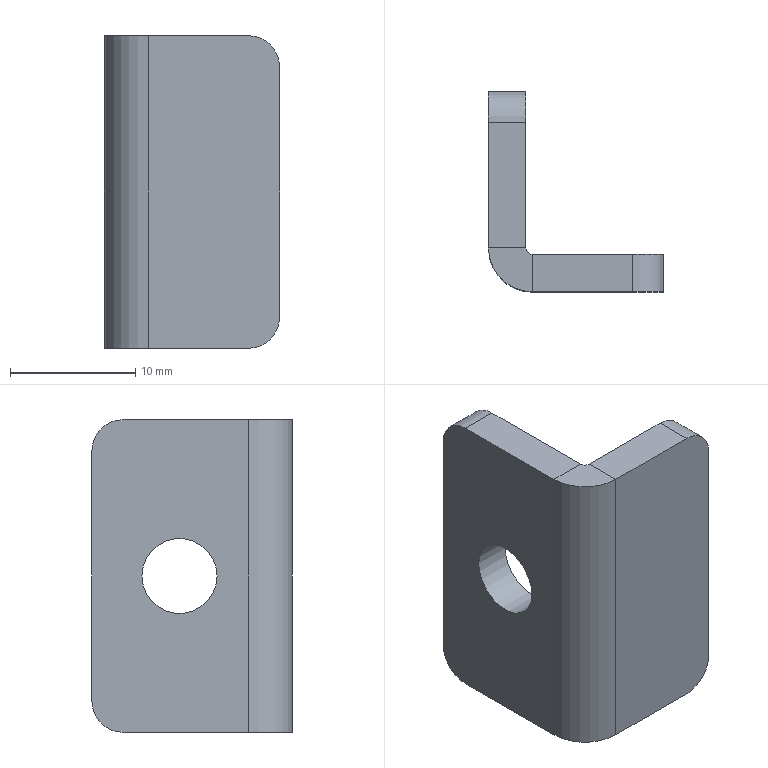Part | STEP file | 6100513 | 1 solid | 19 faces | box 14 x 16 x 25 mm | volume 1860 mm3 | plane 12 | cylinder 7 | commonest cylinder face diameters 5 x4 1 x1 6 x1 7 x1
STEP:
#1=CARTESIAN_POINT('',(0.,0.,0.));
#2=DIRECTION('',(0.,0.,1.));
#3=DIRECTION('',(1.,0.,0.));
#4=AXIS2_PLACEMENT_3D('',#1,#2,#3);
#5=CARTESIAN_POINT('',(0.,3.5,12.5));
#6=VERTEX_POINT('',#5);
#7=CARTESIAN_POINT('',(3.,3.5,12.5));
#8=VERTEX_POINT('',#7);
#9=CARTESIAN_POINT('',(0.,3.5,12.5));
#10=DIRECTION('',(1.,0.,0.));
#11=VECTOR('',#10,1.);
#12=LINE('',#9,#11);
#13=CARTESIAN_POINT('',(0.,3.5,12.5));
#14=DIRECTION('',(0.,0.,1.));
#15=DIRECTION('',(1.,0.,0.));
#16=AXIS2_PLACEMENT_3D('',#13,#14,#15);
#17=PLANE('',#16);
#18=CARTESIAN_POINT('',(0.,0.));
#19=DIRECTION('',(1.,0.));
#20=VECTOR('',#19,1.);
#21=LINE('',#18,#20);
#22=(GEOMETRIC_REPRESENTATION_CONTEXT(2)PARAMETRIC_REPRESENTATION_CONTEXT()REPRESENTATION_CONTEXT('',''));
#23=DEFINITIONAL_REPRESENTATION('',(#21),#22);
#24=PCURVE('',#17,#23);
#25=CARTESIAN_POINT('',(3.5,3.,12.5));
#26=DIRECTION('',(0.,0.,1.));
#27=DIRECTION('',(1.,0.,0.));
#28=AXIS2_PLACEMENT_3D('',#25,#26,#27);
#29=PLANE('',#28);
#30=CARTESIAN_POINT('',(-3.5,0.5));
#31=DIRECTION('',(1.,0.));
#32=VECTOR('',#31,1.);
#33=LINE('',#30,#32);
#34=(GEOMETRIC_REPRESENTATION_CONTEXT(2)PARAMETRIC_REPRESENTATION_CONTEXT()REPRESENTATION_CONTEXT('',''));
#35=DEFINITIONAL_REPRESENTATION('',(#33),#34);
#36=PCURVE('',#29,#35);
#37=SURFACE_CURVE('',#12,(#24,#36),.PCURVE_S1.);
#38=EDGE_CURVE('',#6,#8,#37,.T.);
#39=ORIENTED_EDGE('',*,*,#38,.F.);
#40=CARTESIAN_POINT('',(3.5,0.,12.5));
#41=VERTEX_POINT('',#40);
#42=CARTESIAN_POINT('',(3.5,3.5,12.5));
#43=DIRECTION('',(0.,0.,1.));
#44=DIRECTION('',(-1.,0.,0.));
#45=AXIS2_PLACEMENT_3D('',#42,#43,#44);
#46=CIRCLE('',#45,3.5);
#47=CARTESIAN_POINT('',(3.5,0.));
#48=DIRECTION('',(-1.,0.));
#49=AXIS2_PLACEMENT_2D('',#47,#48);
#50=CIRCLE('',#49,3.5);
#51=(GEOMETRIC_REPRESENTATION_CONTEXT(2)PARAMETRIC_REPRESENTATION_CONTEXT()REPRESENTATION_CONTEXT('',''));
#52=DEFINITIONAL_REPRESENTATION('',(#50),#51);
#53=PCURVE('',#17,#52);
#54=CARTESIAN_POINT('',(3.5,3.5,12.5));
#55=DIRECTION('',(0.,0.,-1.));
#56=DIRECTION('',(-1.,0.,0.));
#57=AXIS2_PLACEMENT_3D('',#54,#55,#56);
#58=CYLINDRICAL_SURFACE('',#57,3.5);
#59=CARTESIAN_POINT('',(6.283,0.));
#60=DIRECTION('',(-1.,0.));
#61=VECTOR('',#60,1.);
#62=LINE('',#59,#61);
#63=(GEOMETRIC_REPRESENTATION_CONTEXT(2)PARAMETRIC_REPRESENTATION_CONTEXT()REPRESENTATION_CONTEXT('',''));
#64=DEFINITIONAL_REPRESENTATION('',(#62),#63);
#65=PCURVE('',#58,#64);
#66=SURFACE_CURVE('',#46,(#53,#65),.PCURVE_S1.);
#67=EDGE_CURVE('',#6,#41,#66,.T.);
#68=ORIENTED_EDGE('',*,*,#67,.T.);
#69=CARTESIAN_POINT('',(3.5,3.,12.5));
#70=VERTEX_POINT('',#69);
#71=CARTESIAN_POINT('',(3.5,3.,12.5));
#72=DIRECTION('',(0.,-1.,0.));
#73=VECTOR('',#72,1.);
#74=LINE('',#71,#73);
#75=CARTESIAN_POINT('',(3.5,-0.5));
#76=DIRECTION('',(0.,-1.));
#77=VECTOR('',#76,1.);
#78=LINE('',#75,#77);
#79=(GEOMETRIC_REPRESENTATION_CONTEXT(2)PARAMETRIC_REPRESENTATION_CONTEXT()REPRESENTATION_CONTEXT('',''));
#80=DEFINITIONAL_REPRESENTATION('',(#78),#79);
#81=PCURVE('',#17,#80);
#82=CARTESIAN_POINT('',(3.5,3.5,12.5));
#83=DIRECTION('',(0.,0.,1.));
#84=DIRECTION('',(1.,0.,0.));
#85=AXIS2_PLACEMENT_3D('',#82,#83,#84);
#86=PLANE('',#85);
#87=CARTESIAN_POINT('',(0.,-0.5));
#88=DIRECTION('',(0.,-1.));
#89=VECTOR('',#88,1.);
#90=LINE('',#87,#89);
#91=(GEOMETRIC_REPRESENTATION_CONTEXT(2)PARAMETRIC_REPRESENTATION_CONTEXT()REPRESENTATION_CONTEXT('',''));
#92=DEFINITIONAL_REPRESENTATION('',(#90),#91);
#93=PCURVE('',#86,#92);
#94=SURFACE_CURVE('',#74,(#81,#93),.PCURVE_S1.);
#95=EDGE_CURVE('',#70,#41,#94,.T.);
#96=ORIENTED_EDGE('',*,*,#95,.F.);
#97=CARTESIAN_POINT('',(3.5,3.5,12.5));
#98=DIRECTION('',(0.,0.,1.));
#99=DIRECTION('',(1.,0.,0.));
#100=AXIS2_PLACEMENT_3D('',#97,#98,#99);
#101=CIRCLE('',#100,0.5);
#102=CARTESIAN_POINT('',(3.5,0.));
#103=DIRECTION('',(1.,0.));
#104=AXIS2_PLACEMENT_2D('',#102,#103);
#105=CIRCLE('',#104,0.5);
#106=(GEOMETRIC_REPRESENTATION_CONTEXT(2)PARAMETRIC_REPRESENTATION_CONTEXT()REPRESENTATION_CONTEXT('',''));
#107=DEFINITIONAL_REPRESENTATION('',(#105),#106);
#108=PCURVE('',#17,#107);
#109=CARTESIAN_POINT('',(3.5,3.5,12.5));
#110=DIRECTION('',(0.,0.,-1.));
#111=DIRECTION('',(-1.,0.,0.));
#112=AXIS2_PLACEMENT_3D('',#109,#110,#111);
#113=CYLINDRICAL_SURFACE('',#112,0.5);
#114=CARTESIAN_POINT('',(9.425,0.));
#115=DIRECTION('',(-1.,0.));
#116=VECTOR('',#115,1.);
#117=LINE('',#114,#116);
#118=(GEOMETRIC_REPRESENTATION_CONTEXT(2)PARAMETRIC_REPRESENTATION_CONTEXT()REPRESENTATION_CONTEXT('',''));
#119=DEFINITIONAL_REPRESENTATION('',(#117),#118);
#120=PCURVE('',#113,#119);
#121=SURFACE_CURVE('',#101,(#108,#120),.PCURVE_S1.);
#122=EDGE_CURVE('',#8,#70,#121,.T.);
#123=ORIENTED_EDGE('',*,*,#122,.F.);
#124=EDGE_LOOP('',(#39,#68,#96,#123));
#125=FACE_BOUND('',#124,.T.);
#126=ADVANCED_FACE('',(#125),#17,.T.);
#127=CARTESIAN_POINT('',(3.,13.5,12.5));
#128=VERTEX_POINT('',#127);
#129=CARTESIAN_POINT('',(3.,16.,12.5));
#130=DIRECTION('',(0.,-1.,0.));
#131=VECTOR('',#130,1.);
#132=LINE('',#129,#131);
#133=CARTESIAN_POINT('',(-0.5,13.));
#134=DIRECTION('',(0.,-1.));
#135=VECTOR('',#134,1.);
#136=LINE('',#133,#135);
#137=(GEOMETRIC_REPRESENTATION_CONTEXT(2)PARAMETRIC_REPRESENTATION_CONTEXT()REPRESENTATION_CONTEXT('',''));
#138=DEFINITIONAL_REPRESENTATION('',(#136),#137);
#139=PCURVE('',#29,#138);
#140=CARTESIAN_POINT('',(3.,16.,12.5));
#141=DIRECTION('',(1.,0.,0.));
#142=DIRECTION('',(0.,1.,0.));
#143=AXIS2_PLACEMENT_3D('',#140,#141,#142);
#144=PLANE('',#143);
#145=CARTESIAN_POINT('',(0.,0.));
#146=DIRECTION('',(-1.,0.));
#147=VECTOR('',#146,1.);
#148=LINE('',#145,#147);
#149=(GEOMETRIC_REPRESENTATION_CONTEXT(2)PARAMETRIC_REPRESENTATION_CONTEXT()REPRESENTATION_CONTEXT('',''));
#150=DEFINITIONAL_REPRESENTATION('',(#148),#149);
#151=PCURVE('',#144,#150);
#152=SURFACE_CURVE('',#132,(#139,#151),.PCURVE_S1.);
#153=EDGE_CURVE('',#128,#8,#152,.T.);
#154=ORIENTED_EDGE('',*,*,#153,.F.);
#155=CARTESIAN_POINT('',(0.,13.5,12.5));
#156=VERTEX_POINT('',#155);
#157=CARTESIAN_POINT('',(3.5,13.5,12.5));
#158=DIRECTION('',(-1.,0.,0.));
#159=VECTOR('',#158,1.);
#160=LINE('',#157,#159);
#161=CARTESIAN_POINT('',(0.,10.5));
#162=DIRECTION('',(-1.,0.));
#163=VECTOR('',#162,1.);
#164=LINE('',#161,#163);
#165=(GEOMETRIC_REPRESENTATION_CONTEXT(2)PARAMETRIC_REPRESENTATION_CONTEXT()REPRESENTATION_CONTEXT('',''));
#166=DEFINITIONAL_REPRESENTATION('',(#164),#165);
#167=PCURVE('',#29,#166);
#168=CARTESIAN_POINT('',(0.,13.5,10.));
#169=DIRECTION('',(1.,0.,0.));
#170=DIRECTION('',(0.,1.,0.));
#171=AXIS2_PLACEMENT_3D('',#168,#169,#170);
#172=CYLINDRICAL_SURFACE('',#171,2.5);
#173=CARTESIAN_POINT('',(1.571,3.5));
#174=DIRECTION('',(0.,-1.));
#175=VECTOR('',#174,1.);
#176=LINE('',#173,#175);
#177=(GEOMETRIC_REPRESENTATION_CONTEXT(2)PARAMETRIC_REPRESENTATION_CONTEXT()REPRESENTATION_CONTEXT('',''));
#178=DEFINITIONAL_REPRESENTATION('',(#176),#177);
#179=PCURVE('',#172,#178);
#180=SURFACE_CURVE('',#160,(#167,#179),.PCURVE_S1.);
#181=EDGE_CURVE('',#128,#156,#180,.T.);
#182=ORIENTED_EDGE('',*,*,#181,.T.);
#183=CARTESIAN_POINT('',(0.,16.,12.5));
#184=DIRECTION('',(0.,-1.,0.));
#185=VECTOR('',#184,1.);
#186=LINE('',#183,#185);
#187=CARTESIAN_POINT('',(-3.5,13.));
#188=DIRECTION('',(0.,-1.));
#189=VECTOR('',#188,1.);
#190=LINE('',#187,#189);
#191=(GEOMETRIC_REPRESENTATION_CONTEXT(2)PARAMETRIC_REPRESENTATION_CONTEXT()REPRESENTATION_CONTEXT('',''));
#192=DEFINITIONAL_REPRESENTATION('',(#190),#191);
#193=PCURVE('',#29,#192);
#194=CARTESIAN_POINT('',(0.,16.,12.5));
#195=DIRECTION('',(1.,0.,0.));
#196=DIRECTION('',(0.,1.,0.));
#197=AXIS2_PLACEMENT_3D('',#194,#195,#196);
#198=PLANE('',#197);
#199=CARTESIAN_POINT('',(0.,0.));
#200=DIRECTION('',(-1.,0.));
#201=VECTOR('',#200,1.);
#202=LINE('',#199,#201);
#203=(GEOMETRIC_REPRESENTATION_CONTEXT(2)PARAMETRIC_REPRESENTATION_CONTEXT()REPRESENTATION_CONTEXT('',''));
#204=DEFINITIONAL_REPRESENTATION('',(#202),#203);
#205=PCURVE('',#198,#204);
#206=SURFACE_CURVE('',#186,(#193,#205),.PCURVE_S1.);
#207=EDGE_CURVE('',#156,#6,#206,.T.);
#208=ORIENTED_EDGE('',*,*,#207,.T.);
#209=ORIENTED_EDGE('',*,*,#38,.T.);
#210=EDGE_LOOP('',(#154,#182,#208,#209));
#211=FACE_BOUND('',#210,.T.);
#212=ADVANCED_FACE('',(#211),#29,.T.);
#213=CARTESIAN_POINT('',(3.5,0.,-12.5));
#214=VERTEX_POINT('',#213);
#215=CARTESIAN_POINT('',(3.5,3.,-12.5));
#216=VERTEX_POINT('',#215);
#217=CARTESIAN_POINT('',(3.5,0.,-12.5));
#218=DIRECTION('',(0.,1.,0.));
#219=VECTOR('',#218,1.);
#220=LINE('',#217,#219);
#221=CARTESIAN_POINT('',(3.5,0.,-12.5));
#222=DIRECTION('',(0.,0.,-1.));
#223=DIRECTION('',(-1.,0.,0.));
#224=AXIS2_PLACEMENT_3D('',#221,#222,#223);
#225=PLANE('',#224);
#226=CARTESIAN_POINT('',(0.,0.));
#227=DIRECTION('',(0.,1.));
#228=VECTOR('',#227,1.);
#229=LINE('',#226,#228);
#230=(GEOMETRIC_REPRESENTATION_CONTEXT(2)PARAMETRIC_REPRESENTATION_CONTEXT()REPRESENTATION_CONTEXT('',''));
#231=DEFINITIONAL_REPRESENTATION('',(#229),#230);
#232=PCURVE('',#225,#231);
#233=CARTESIAN_POINT('',(3.,3.5,-12.5));
#234=DIRECTION('',(0.,0.,-1.));
#235=DIRECTION('',(-1.,0.,0.));
#236=AXIS2_PLACEMENT_3D('',#233,#234,#235);
#237=PLANE('',#236);
#238=CARTESIAN_POINT('',(-0.5,-3.5));
#239=DIRECTION('',(0.,1.));
#240=VECTOR('',#239,1.);
#241=LINE('',#238,#240);
#242=(GEOMETRIC_REPRESENTATION_CONTEXT(2)PARAMETRIC_REPRESENTATION_CONTEXT()REPRESENTATION_CONTEXT('',''));
#243=DEFINITIONAL_REPRESENTATION('',(#241),#242);
#244=PCURVE('',#237,#243);
#245=SURFACE_CURVE('',#220,(#232,#244),.PCURVE_S1.);
#246=EDGE_CURVE('',#214,#216,#245,.T.);
#247=ORIENTED_EDGE('',*,*,#246,.F.);
#248=CARTESIAN_POINT('',(0.,3.5,-12.5));
#249=VERTEX_POINT('',#248);
#250=CARTESIAN_POINT('',(3.5,3.5,-12.5));
#251=DIRECTION('',(0.,0.,1.));
#252=DIRECTION('',(-1.,0.,0.));
#253=AXIS2_PLACEMENT_3D('',#250,#251,#252);
#254=CIRCLE('',#253,3.5);
#255=CARTESIAN_POINT('',(3.5,3.5));
#256=CARTESIAN_POINT('',(3.5,-2.562));
#257=CARTESIAN_POINT('',(-1.75,0.4689));
#258=CARTESIAN_POINT('',(-7.,3.5));
#259=CARTESIAN_POINT('',(-1.75,6.531));
#260=CARTESIAN_POINT('',(3.5,9.562));
#261=CARTESIAN_POINT('',(3.5,3.5));
#262=(BOUNDED_CURVE()B_SPLINE_CURVE(2,(#255,#256,#257,#258,#259,#260,#261),.UNSPECIFIED.,.T.,.F.)B_SPLINE_CURVE_WITH_KNOTS((1,2,2,2,2,1),(-2.094,0.,2.094,4.189,6.283,8.378),.UNSPECIFIED.)CURVE()GEOMETRIC_REPRESENTATION_ITEM()RATIONAL_B_SPLINE_CURVE((1.,0.5,1.,0.5,1.,0.5,1.))REPRESENTATION_ITEM(''));
#263=(GEOMETRIC_REPRESENTATION_CONTEXT(2)PARAMETRIC_REPRESENTATION_CONTEXT()REPRESENTATION_CONTEXT('',''));
#264=DEFINITIONAL_REPRESENTATION('',(#262),#263);
#265=PCURVE('',#225,#264);
#266=CARTESIAN_POINT('',(6.283,25.));
#267=DIRECTION('',(-1.,0.));
#268=VECTOR('',#267,1.);
#269=LINE('',#266,#268);
#270=(GEOMETRIC_REPRESENTATION_CONTEXT(2)PARAMETRIC_REPRESENTATION_CONTEXT()REPRESENTATION_CONTEXT('',''));
#271=DEFINITIONAL_REPRESENTATION('',(#269),#270);
#272=PCURVE('',#58,#271);
#273=SURFACE_CURVE('',#254,(#265,#272),.PCURVE_S1.);
#274=EDGE_CURVE('',#249,#214,#273,.T.);
#275=ORIENTED_EDGE('',*,*,#274,.F.);
#276=CARTESIAN_POINT('',(3.,3.5,-12.5));
#277=VERTEX_POINT('',#276);
#278=CARTESIAN_POINT('',(3.,3.5,-12.5));
#279=DIRECTION('',(-1.,0.,0.));
#280=VECTOR('',#279,1.);
#281=LINE('',#278,#280);
#282=CARTESIAN_POINT('',(0.5,3.5));
#283=DIRECTION('',(1.,0.));
#284=VECTOR('',#283,1.);
#285=LINE('',#282,#284);
#286=(GEOMETRIC_REPRESENTATION_CONTEXT(2)PARAMETRIC_REPRESENTATION_CONTEXT()REPRESENTATION_CONTEXT('',''));
#287=DEFINITIONAL_REPRESENTATION('',(#285),#286);
#288=PCURVE('',#225,#287);
#289=CARTESIAN_POINT('',(3.5,3.5,-12.5));
#290=DIRECTION('',(0.,0.,1.));
#291=DIRECTION('',(1.,0.,0.));
#292=AXIS2_PLACEMENT_3D('',#289,#290,#291);
#293=PLANE('',#292);
#294=CARTESIAN_POINT('',(-0.5,0.));
#295=DIRECTION('',(-1.,0.));
#296=VECTOR('',#295,1.);
#297=LINE('',#294,#296);
#298=(GEOMETRIC_REPRESENTATION_CONTEXT(2)PARAMETRIC_REPRESENTATION_CONTEXT()REPRESENTATION_CONTEXT('',''));
#299=DEFINITIONAL_REPRESENTATION('',(#297),#298);
#300=PCURVE('',#293,#299);
#301=SURFACE_CURVE('',#281,(#288,#300),.PCURVE_S1.);
#302=EDGE_CURVE('',#277,#249,#301,.T.);
#303=ORIENTED_EDGE('',*,*,#302,.F.);
#304=CARTESIAN_POINT('',(3.5,3.5,-12.5));
#305=DIRECTION('',(0.,0.,1.));
#306=DIRECTION('',(1.,0.,0.));
#307=AXIS2_PLACEMENT_3D('',#304,#305,#306);
#308=CIRCLE('',#307,0.5);
#309=CARTESIAN_POINT('',(-0.5,3.5));
#310=CARTESIAN_POINT('',(-0.5,4.366));
#311=CARTESIAN_POINT('',(0.25,3.933));
#312=CARTESIAN_POINT('',(1.,3.5));
#313=CARTESIAN_POINT('',(0.25,3.067));
#314=CARTESIAN_POINT('',(-0.5,2.634));
#315=CARTESIAN_POINT('',(-0.5,3.5));
#316=(BOUNDED_CURVE()B_SPLINE_CURVE(2,(#309,#310,#311,#312,#313,#314,#315),.UNSPECIFIED.,.T.,.F.)B_SPLINE_CURVE_WITH_KNOTS((1,2,2,2,2,1),(-2.094,0.,2.094,4.189,6.283,8.378),.UNSPECIFIED.)CURVE()GEOMETRIC_REPRESENTATION_ITEM()RATIONAL_B_SPLINE_CURVE((1.,0.5,1.,0.5,1.,0.5,1.))REPRESENTATION_ITEM(''));
#317=(GEOMETRIC_REPRESENTATION_CONTEXT(2)PARAMETRIC_REPRESENTATION_CONTEXT()REPRESENTATION_CONTEXT('',''));
#318=DEFINITIONAL_REPRESENTATION('',(#316),#317);
#319=PCURVE('',#225,#318);
#320=CARTESIAN_POINT('',(9.425,25.));
#321=DIRECTION('',(-1.,0.));
#322=VECTOR('',#321,1.);
#323=LINE('',#320,#322);
#324=(GEOMETRIC_REPRESENTATION_CONTEXT(2)PARAMETRIC_REPRESENTATION_CONTEXT()REPRESENTATION_CONTEXT('',''));
#325=DEFINITIONAL_REPRESENTATION('',(#323),#324);
#326=PCURVE('',#113,#325);
#327=SURFACE_CURVE('',#308,(#319,#326),.PCURVE_S1.);
#328=EDGE_CURVE('',#277,#216,#327,.T.);
#329=ORIENTED_EDGE('',*,*,#328,.T.);
#330=EDGE_LOOP('',(#247,#275,#303,#329));
#331=FACE_BOUND('',#330,.T.);
#332=ADVANCED_FACE('',(#331),#225,.T.);
#333=CARTESIAN_POINT('',(11.5,3.,-12.5));
#334=VERTEX_POINT('',#333);
#335=CARTESIAN_POINT('',(3.5,3.,-12.5));
#336=DIRECTION('',(1.,0.,0.));
#337=VECTOR('',#336,1.);
#338=LINE('',#335,#337);
#339=CARTESIAN_POINT('',(-0.5,-0.5));
#340=DIRECTION('',(-1.,0.));
#341=VECTOR('',#340,1.);
#342=LINE('',#339,#341);
#343=(GEOMETRIC_REPRESENTATION_CONTEXT(2)PARAMETRIC_REPRESENTATION_CONTEXT()REPRESENTATION_CONTEXT('',''));
#344=DEFINITIONAL_REPRESENTATION('',(#342),#343);
#345=PCURVE('',#237,#344);
#346=CARTESIAN_POINT('',(3.5,3.,12.5));
#347=DIRECTION('',(0.,1.,0.));
#348=DIRECTION('',(0.,0.,1.));
#349=AXIS2_PLACEMENT_3D('',#346,#347,#348);
#350=PLANE('',#349);
#351=CARTESIAN_POINT('',(-25.,0.));
#352=DIRECTION('',(0.,1.));
#353=VECTOR('',#352,1.);
#354=LINE('',#351,#353);
#355=(GEOMETRIC_REPRESENTATION_CONTEXT(2)PARAMETRIC_REPRESENTATION_CONTEXT()REPRESENTATION_CONTEXT('',''));
#356=DEFINITIONAL_REPRESENTATION('',(#354),#355);
#357=PCURVE('',#350,#356);
#358=SURFACE_CURVE('',#338,(#345,#357),.PCURVE_S1.);
#359=EDGE_CURVE('',#216,#334,#358,.T.);
#360=ORIENTED_EDGE('',*,*,#359,.T.);
#361=CARTESIAN_POINT('',(11.5,0.,-12.5));
#362=VERTEX_POINT('',#361);
#363=CARTESIAN_POINT('',(11.5,3.5,-12.5));
#364=DIRECTION('',(0.,-1.,0.));
#365=VECTOR('',#364,1.);
#366=LINE('',#363,#365);
#367=CARTESIAN_POINT('',(-8.5,0.));
#368=DIRECTION('',(0.,-1.));
#369=VECTOR('',#368,1.);
#370=LINE('',#367,#369);
#371=(GEOMETRIC_REPRESENTATION_CONTEXT(2)PARAMETRIC_REPRESENTATION_CONTEXT()REPRESENTATION_CONTEXT('',''));
#372=DEFINITIONAL_REPRESENTATION('',(#370),#371);
#373=PCURVE('',#237,#372);
#374=CARTESIAN_POINT('',(11.5,3.5,-10.));
#375=DIRECTION('',(0.,-1.,0.));
#376=DIRECTION('',(0.,0.,-1.));
#377=AXIS2_PLACEMENT_3D('',#374,#375,#376);
#378=CYLINDRICAL_SURFACE('',#377,2.5);
#379=CARTESIAN_POINT('',(0.,0.));
#380=DIRECTION('',(0.,1.));
#381=VECTOR('',#380,1.);
#382=LINE('',#379,#381);
#383=(GEOMETRIC_REPRESENTATION_CONTEXT(2)PARAMETRIC_REPRESENTATION_CONTEXT()REPRESENTATION_CONTEXT('',''));
#384=DEFINITIONAL_REPRESENTATION('',(#382),#383);
#385=PCURVE('',#378,#384);
#386=SURFACE_CURVE('',#366,(#373,#385),.PCURVE_S1.);
#387=EDGE_CURVE('',#334,#362,#386,.T.);
#388=ORIENTED_EDGE('',*,*,#387,.T.);
#389=CARTESIAN_POINT('',(3.5,0.,-12.5));
#390=DIRECTION('',(1.,0.,0.));
#391=VECTOR('',#390,1.);
#392=LINE('',#389,#391);
#393=CARTESIAN_POINT('',(-0.5,-3.5));
#394=DIRECTION('',(-1.,0.));
#395=VECTOR('',#394,1.);
#396=LINE('',#393,#395);
#397=(GEOMETRIC_REPRESENTATION_CONTEXT(2)PARAMETRIC_REPRESENTATION_CONTEXT()REPRESENTATION_CONTEXT('',''));
#398=DEFINITIONAL_REPRESENTATION('',(#396),#397);
#399=PCURVE('',#237,#398);
#400=CARTESIAN_POINT('',(3.5,0.,12.5));
#401=DIRECTION('',(0.,1.,0.));
#402=DIRECTION('',(0.,0.,1.));
#403=AXIS2_PLACEMENT_3D('',#400,#401,#402);
#404=PLANE('',#403);
#405=CARTESIAN_POINT('',(-25.,0.));
#406=DIRECTION('',(0.,1.));
#407=VECTOR('',#406,1.);
#408=LINE('',#405,#407);
#409=(GEOMETRIC_REPRESENTATION_CONTEXT(2)PARAMETRIC_REPRESENTATION_CONTEXT()REPRESENTATION_CONTEXT('',''));
#410=DEFINITIONAL_REPRESENTATION('',(#408),#409);
#411=PCURVE('',#404,#410);
#412=SURFACE_CURVE('',#392,(#399,#411),.PCURVE_S1.);
#413=EDGE_CURVE('',#214,#362,#412,.T.);
#414=ORIENTED_EDGE('',*,*,#413,.F.);
#415=ORIENTED_EDGE('',*,*,#246,.T.);
#416=EDGE_LOOP('',(#360,#388,#414,#415));
#417=FACE_BOUND('',#416,.T.);
#418=ADVANCED_FACE('',(#417),#237,.T.);
#419=ORIENTED_EDGE('',*,*,#413,.T.);
#420=CARTESIAN_POINT('',(14.,0.,-10.));
#421=VERTEX_POINT('',#420);
#422=CARTESIAN_POINT('',(11.5,0.,-10.));
#423=DIRECTION('',(0.,-1.,0.));
#424=DIRECTION('',(0.,0.,1.));
#425=AXIS2_PLACEMENT_3D('',#422,#423,#424);
#426=CIRCLE('',#425,2.5);
#427=CARTESIAN_POINT('',(-20.,8.));
#428=CARTESIAN_POINT('',(-20.,3.67));
#429=CARTESIAN_POINT('',(-23.75,5.835));
#430=CARTESIAN_POINT('',(-27.5,8.));
#431=CARTESIAN_POINT('',(-23.75,10.165));
#432=CARTESIAN_POINT('',(-20.,12.33));
#433=CARTESIAN_POINT('',(-20.,8.));
#434=(BOUNDED_CURVE()B_SPLINE_CURVE(2,(#427,#428,#429,#430,#431,#432,#433),.UNSPECIFIED.,.T.,.F.)B_SPLINE_CURVE_WITH_KNOTS((1,2,2,2,2,1),(-2.094,0.,2.094,4.189,6.283,8.378),.UNSPECIFIED.)CURVE()GEOMETRIC_REPRESENTATION_ITEM()RATIONAL_B_SPLINE_CURVE((1.,0.5,1.,0.5,1.,0.5,1.))REPRESENTATION_ITEM(''));
#435=(GEOMETRIC_REPRESENTATION_CONTEXT(2)PARAMETRIC_REPRESENTATION_CONTEXT()REPRESENTATION_CONTEXT('',''));
#436=DEFINITIONAL_REPRESENTATION('',(#434),#435);
#437=PCURVE('',#404,#436);
#438=CARTESIAN_POINT('',(-3.142,3.5));
#439=DIRECTION('',(1.,0.));
#440=VECTOR('',#439,1.);
#441=LINE('',#438,#440);
#442=(GEOMETRIC_REPRESENTATION_CONTEXT(2)PARAMETRIC_REPRESENTATION_CONTEXT()REPRESENTATION_CONTEXT('',''));
#443=DEFINITIONAL_REPRESENTATION('',(#441),#442);
#444=PCURVE('',#378,#443);
#445=SURFACE_CURVE('',#426,(#437,#444),.PCURVE_S1.);
#446=EDGE_CURVE('',#362,#421,#445,.T.);
#447=ORIENTED_EDGE('',*,*,#446,.T.);
#448=CARTESIAN_POINT('',(14.,0.,10.));
#449=VERTEX_POINT('',#448);
#450=CARTESIAN_POINT('',(14.,0.,12.5));
#451=DIRECTION('',(0.,0.,-1.));
#452=VECTOR('',#451,1.);
#453=LINE('',#450,#452);
#454=CARTESIAN_POINT('',(0.,10.5));
#455=DIRECTION('',(-1.,0.));
#456=VECTOR('',#455,1.);
#457=LINE('',#454,#456);
#458=(GEOMETRIC_REPRESENTATION_CONTEXT(2)PARAMETRIC_REPRESENTATION_CONTEXT()REPRESENTATION_CONTEXT('',''));
#459=DEFINITIONAL_REPRESENTATION('',(#457),#458);
#460=PCURVE('',#404,#459);
#461=CARTESIAN_POINT('',(14.,3.,12.5));
#462=DIRECTION('',(1.,0.,0.));
#463=DIRECTION('',(0.,0.,-1.));
#464=AXIS2_PLACEMENT_3D('',#461,#462,#463);
#465=PLANE('',#464);
#466=CARTESIAN_POINT('',(0.,-3.));
#467=DIRECTION('',(1.,0.));
#468=VECTOR('',#467,1.);
#469=LINE('',#466,#468);
#470=(GEOMETRIC_REPRESENTATION_CONTEXT(2)PARAMETRIC_REPRESENTATION_CONTEXT()REPRESENTATION_CONTEXT('',''));
#471=DEFINITIONAL_REPRESENTATION('',(#469),#470);
#472=PCURVE('',#465,#471);
#473=SURFACE_CURVE('',#453,(#460,#472),.PCURVE_S1.);
#474=EDGE_CURVE('',#449,#421,#473,.T.);
#475=ORIENTED_EDGE('',*,*,#474,.F.);
#476=CARTESIAN_POINT('',(11.5,0.,12.5));
#477=VERTEX_POINT('',#476);
#478=CARTESIAN_POINT('',(11.5,0.,10.));
#479=DIRECTION('',(0.,-1.,0.));
#480=DIRECTION('',(0.,0.,1.));
#481=AXIS2_PLACEMENT_3D('',#478,#479,#480);
#482=CIRCLE('',#481,2.5);
#483=CARTESIAN_POINT('',(0.,8.));
#484=CARTESIAN_POINT('',(0.,3.67));
#485=CARTESIAN_POINT('',(-3.75,5.835));
#486=CARTESIAN_POINT('',(-7.5,8.));
#487=CARTESIAN_POINT('',(-3.75,10.165));
#488=CARTESIAN_POINT('',(0.,12.33));
#489=CARTESIAN_POINT('',(0.,8.));
#490=(BOUNDED_CURVE()B_SPLINE_CURVE(2,(#483,#484,#485,#486,#487,#488,#489),.UNSPECIFIED.,.T.,.F.)B_SPLINE_CURVE_WITH_KNOTS((1,2,2,2,2,1),(-2.094,0.,2.094,4.189,6.283,8.378),.UNSPECIFIED.)CURVE()GEOMETRIC_REPRESENTATION_ITEM()RATIONAL_B_SPLINE_CURVE((1.,0.5,1.,0.5,1.,0.5,1.))REPRESENTATION_ITEM(''));
#491=(GEOMETRIC_REPRESENTATION_CONTEXT(2)PARAMETRIC_REPRESENTATION_CONTEXT()REPRESENTATION_CONTEXT('',''));
#492=DEFINITIONAL_REPRESENTATION('',(#490),#491);
#493=PCURVE('',#404,#492);
#494=CARTESIAN_POINT('',(11.5,3.,10.));
#495=DIRECTION('',(0.,-1.,0.));
#496=DIRECTION('',(0.,0.,-1.));
#497=AXIS2_PLACEMENT_3D('',#494,#495,#496);
#498=CYLINDRICAL_SURFACE('',#497,2.5);
#499=CARTESIAN_POINT('',(-3.142,3.));
#500=DIRECTION('',(1.,0.));
#501=VECTOR('',#500,1.);
#502=LINE('',#499,#501);
#503=(GEOMETRIC_REPRESENTATION_CONTEXT(2)PARAMETRIC_REPRESENTATION_CONTEXT()REPRESENTATION_CONTEXT('',''));
#504=DEFINITIONAL_REPRESENTATION('',(#502),#503);
#505=PCURVE('',#498,#504);
#506=SURFACE_CURVE('',#482,(#493,#505),.PCURVE_S1.);
#507=EDGE_CURVE('',#449,#477,#506,.T.);
#508=ORIENTED_EDGE('',*,*,#507,.T.);
#509=CARTESIAN_POINT('',(3.5,0.,12.5));
#510=DIRECTION('',(1.,0.,0.));
#511=VECTOR('',#510,1.);
#512=LINE('',#509,#511);
#513=CARTESIAN_POINT('',(0.,0.));
#514=DIRECTION('',(0.,1.));
#515=VECTOR('',#514,1.);
#516=LINE('',#513,#515);
#517=(GEOMETRIC_REPRESENTATION_CONTEXT(2)PARAMETRIC_REPRESENTATION_CONTEXT()REPRESENTATION_CONTEXT('',''));
#518=DEFINITIONAL_REPRESENTATION('',(#516),#517);
#519=PCURVE('',#404,#518);
#520=CARTESIAN_POINT('',(0.,-3.5));
#521=DIRECTION('',(1.,0.));
#522=VECTOR('',#521,1.);
#523=LINE('',#520,#522);
#524=(GEOMETRIC_REPRESENTATION_CONTEXT(2)PARAMETRIC_REPRESENTATION_CONTEXT()REPRESENTATION_CONTEXT('',''));
#525=DEFINITIONAL_REPRESENTATION('',(#523),#524);
#526=PCURVE('',#86,#525);
#527=SURFACE_CURVE('',#512,(#519,#526),.PCURVE_S1.);
#528=EDGE_CURVE('',#41,#477,#527,.T.);
#529=ORIENTED_EDGE('',*,*,#528,.F.);
#530=CARTESIAN_POINT('',(3.5,0.,12.5));
#531=DIRECTION('',(0.,0.,-1.));
#532=VECTOR('',#531,1.);
#533=LINE('',#530,#532);
#534=CARTESIAN_POINT('',(0.,0.));
#535=DIRECTION('',(-1.,0.));
#536=VECTOR('',#535,1.);
#537=LINE('',#534,#536);
#538=(GEOMETRIC_REPRESENTATION_CONTEXT(2)PARAMETRIC_REPRESENTATION_CONTEXT()REPRESENTATION_CONTEXT('',''));
#539=DEFINITIONAL_REPRESENTATION('',(#537),#538);
#540=PCURVE('',#404,#539);
#541=CARTESIAN_POINT('',(4.712,0.));
#542=DIRECTION('',(0.,1.));
#543=VECTOR('',#542,1.);
#544=LINE('',#541,#543);
#545=(GEOMETRIC_REPRESENTATION_CONTEXT(2)PARAMETRIC_REPRESENTATION_CONTEXT()REPRESENTATION_CONTEXT('',''));
#546=DEFINITIONAL_REPRESENTATION('',(#544),#545);
#547=PCURVE('',#58,#546);
#548=SURFACE_CURVE('',#533,(#540,#547),.PCURVE_S1.);
#549=EDGE_CURVE('',#41,#214,#548,.T.);
#550=ORIENTED_EDGE('',*,*,#549,.T.);
#551=EDGE_LOOP('',(#419,#447,#475,#508,#529,#550));
#552=FACE_BOUND('',#551,.T.);
#553=ADVANCED_FACE('',(#552),#404,.F.);
#554=ORIENTED_EDGE('',*,*,#474,.T.);
#555=CARTESIAN_POINT('',(14.,3.,-10.));
#556=VERTEX_POINT('',#555);
#557=CARTESIAN_POINT('',(14.,3.,-10.));
#558=DIRECTION('',(0.,1.,0.));
#559=VECTOR('',#558,1.);
#560=LINE('',#557,#559);
#561=CARTESIAN_POINT('',(22.5,0.));
#562=DIRECTION('',(0.,1.));
#563=VECTOR('',#562,1.);
#564=LINE('',#561,#563);
#565=(GEOMETRIC_REPRESENTATION_CONTEXT(2)PARAMETRIC_REPRESENTATION_CONTEXT()REPRESENTATION_CONTEXT('',''));
#566=DEFINITIONAL_REPRESENTATION('',(#564),#565);
#567=PCURVE('',#465,#566);
#568=CARTESIAN_POINT('',(1.571,0.5));
#569=DIRECTION('',(0.,-1.));
#570=VECTOR('',#569,1.);
#571=LINE('',#568,#570);
#572=(GEOMETRIC_REPRESENTATION_CONTEXT(2)PARAMETRIC_REPRESENTATION_CONTEXT()REPRESENTATION_CONTEXT('',''));
#573=DEFINITIONAL_REPRESENTATION('',(#571),#572);
#574=PCURVE('',#378,#573);
#575=SURFACE_CURVE('',#560,(#567,#574),.PCURVE_S1.);
#576=EDGE_CURVE('',#421,#556,#575,.T.);
#577=ORIENTED_EDGE('',*,*,#576,.T.);
#578=CARTESIAN_POINT('',(14.,3.,10.));
#579=VERTEX_POINT('',#578);
#580=CARTESIAN_POINT('',(14.,3.,12.5));
#581=DIRECTION('',(0.,0.,-1.));
#582=VECTOR('',#581,1.);
#583=LINE('',#580,#582);
#584=CARTESIAN_POINT('',(0.,0.));
#585=DIRECTION('',(1.,0.));
#586=VECTOR('',#585,1.);
#587=LINE('',#584,#586);
#588=(GEOMETRIC_REPRESENTATION_CONTEXT(2)PARAMETRIC_REPRESENTATION_CONTEXT()REPRESENTATION_CONTEXT('',''));
#589=DEFINITIONAL_REPRESENTATION('',(#587),#588);
#590=PCURVE('',#465,#589);
#591=CARTESIAN_POINT('',(0.,10.5));
#592=DIRECTION('',(-1.,0.));
#593=VECTOR('',#592,1.);
#594=LINE('',#591,#593);
#595=(GEOMETRIC_REPRESENTATION_CONTEXT(2)PARAMETRIC_REPRESENTATION_CONTEXT()REPRESENTATION_CONTEXT('',''));
#596=DEFINITIONAL_REPRESENTATION('',(#594),#595);
#597=PCURVE('',#350,#596);
#598=SURFACE_CURVE('',#583,(#590,#597),.PCURVE_S1.);
#599=EDGE_CURVE('',#579,#556,#598,.T.);
#600=ORIENTED_EDGE('',*,*,#599,.F.);
#601=CARTESIAN_POINT('',(14.,3.,10.));
#602=DIRECTION('',(0.,-1.,0.));
#603=VECTOR('',#602,1.);
#604=LINE('',#601,#603);
#605=CARTESIAN_POINT('',(2.5,0.));
#606=DIRECTION('',(0.,-1.));
#607=VECTOR('',#606,1.);
#608=LINE('',#605,#607);
#609=(GEOMETRIC_REPRESENTATION_CONTEXT(2)PARAMETRIC_REPRESENTATION_CONTEXT()REPRESENTATION_CONTEXT('',''));
#610=DEFINITIONAL_REPRESENTATION('',(#608),#609);
#611=PCURVE('',#465,#610);
#612=CARTESIAN_POINT('',(1.571,0.));
#613=DIRECTION('',(0.,1.));
#614=VECTOR('',#613,1.);
#615=LINE('',#612,#614);
#616=(GEOMETRIC_REPRESENTATION_CONTEXT(2)PARAMETRIC_REPRESENTATION_CONTEXT()REPRESENTATION_CONTEXT('',''));
#617=DEFINITIONAL_REPRESENTATION('',(#615),#616);
#618=PCURVE('',#498,#617);
#619=SURFACE_CURVE('',#604,(#611,#618),.PCURVE_S1.);
#620=EDGE_CURVE('',#579,#449,#619,.T.);
#621=ORIENTED_EDGE('',*,*,#620,.T.);
#622=EDGE_LOOP('',(#554,#577,#600,#621));
#623=FACE_BOUND('',#622,.T.);
#624=ADVANCED_FACE('',(#623),#465,.T.);
#625=ORIENTED_EDGE('',*,*,#599,.T.);
#626=CARTESIAN_POINT('',(11.5,3.,-10.));
#627=DIRECTION('',(0.,1.,0.));
#628=DIRECTION('',(0.,0.,1.));
#629=AXIS2_PLACEMENT_3D('',#626,#627,#628);
#630=CIRCLE('',#629,2.5);
#631=CARTESIAN_POINT('',(-22.5,8.));
#632=DIRECTION('',(1.,0.));
#633=AXIS2_PLACEMENT_2D('',#631,#632);
#634=CIRCLE('',#633,2.5);
#635=(GEOMETRIC_REPRESENTATION_CONTEXT(2)PARAMETRIC_REPRESENTATION_CONTEXT()REPRESENTATION_CONTEXT('',''));
#636=DEFINITIONAL_REPRESENTATION('',(#634),#635);
#637=PCURVE('',#350,#636);
#638=CARTESIAN_POINT('',(3.142,0.5));
#639=DIRECTION('',(-1.,0.));
#640=VECTOR('',#639,1.);
#641=LINE('',#638,#640);
#642=(GEOMETRIC_REPRESENTATION_CONTEXT(2)PARAMETRIC_REPRESENTATION_CONTEXT()REPRESENTATION_CONTEXT('',''));
#643=DEFINITIONAL_REPRESENTATION('',(#641),#642);
#644=PCURVE('',#378,#643);
#645=SURFACE_CURVE('',#630,(#637,#644),.PCURVE_S1.);
#646=EDGE_CURVE('',#556,#334,#645,.T.);
#647=ORIENTED_EDGE('',*,*,#646,.T.);
#648=ORIENTED_EDGE('',*,*,#359,.F.);
#649=CARTESIAN_POINT('',(3.5,3.,12.5));
#650=DIRECTION('',(0.,0.,-1.));
#651=VECTOR('',#650,1.);
#652=LINE('',#649,#651);
#653=CARTESIAN_POINT('',(0.,0.));
#654=DIRECTION('',(-1.,0.));
#655=VECTOR('',#654,1.);
#656=LINE('',#653,#655);
#657=(GEOMETRIC_REPRESENTATION_CONTEXT(2)PARAMETRIC_REPRESENTATION_CONTEXT()REPRESENTATION_CONTEXT('',''));
#658=DEFINITIONAL_REPRESENTATION('',(#656),#657);
#659=PCURVE('',#350,#658);
#660=CARTESIAN_POINT('',(4.712,0.));
#661=DIRECTION('',(0.,1.));
#662=VECTOR('',#661,1.);
#663=LINE('',#660,#662);
#664=(GEOMETRIC_REPRESENTATION_CONTEXT(2)PARAMETRIC_REPRESENTATION_CONTEXT()REPRESENTATION_CONTEXT('',''));
#665=DEFINITIONAL_REPRESENTATION('',(#663),#664);
#666=PCURVE('',#113,#665);
#667=SURFACE_CURVE('',#652,(#659,#666),.PCURVE_S1.);
#668=EDGE_CURVE('',#70,#216,#667,.T.);
#669=ORIENTED_EDGE('',*,*,#668,.F.);
#670=CARTESIAN_POINT('',(11.5,3.,12.5));
#671=VERTEX_POINT('',#670);
#672=CARTESIAN_POINT('',(3.5,3.,12.5));
#673=DIRECTION('',(1.,0.,0.));
#674=VECTOR('',#673,1.);
#675=LINE('',#672,#674);
#676=CARTESIAN_POINT('',(0.,0.));
#677=DIRECTION('',(0.,1.));
#678=VECTOR('',#677,1.);
#679=LINE('',#676,#678);
#680=(GEOMETRIC_REPRESENTATION_CONTEXT(2)PARAMETRIC_REPRESENTATION_CONTEXT()REPRESENTATION_CONTEXT('',''));
#681=DEFINITIONAL_REPRESENTATION('',(#679),#680);
#682=PCURVE('',#350,#681);
#683=CARTESIAN_POINT('',(0.,-0.5));
#684=DIRECTION('',(1.,0.));
#685=VECTOR('',#684,1.);
#686=LINE('',#683,#685);
#687=(GEOMETRIC_REPRESENTATION_CONTEXT(2)PARAMETRIC_REPRESENTATION_CONTEXT()REPRESENTATION_CONTEXT('',''));
#688=DEFINITIONAL_REPRESENTATION('',(#686),#687);
#689=PCURVE('',#86,#688);
#690=SURFACE_CURVE('',#675,(#682,#689),.PCURVE_S1.);
#691=EDGE_CURVE('',#70,#671,#690,.T.);
#692=ORIENTED_EDGE('',*,*,#691,.T.);
#693=CARTESIAN_POINT('',(11.5,3.,10.));
#694=DIRECTION('',(0.,1.,0.));
#695=DIRECTION('',(0.,0.,1.));
#696=AXIS2_PLACEMENT_3D('',#693,#694,#695);
#697=CIRCLE('',#696,2.5);
#698=CARTESIAN_POINT('',(-2.5,8.));
#699=DIRECTION('',(1.,0.));
#700=AXIS2_PLACEMENT_2D('',#698,#699);
#701=CIRCLE('',#700,2.5);
#702=(GEOMETRIC_REPRESENTATION_CONTEXT(2)PARAMETRIC_REPRESENTATION_CONTEXT()REPRESENTATION_CONTEXT('',''));
#703=DEFINITIONAL_REPRESENTATION('',(#701),#702);
#704=PCURVE('',#350,#703);
#705=CARTESIAN_POINT('',(3.142,0.));
#706=DIRECTION('',(-1.,0.));
#707=VECTOR('',#706,1.);
#708=LINE('',#705,#707);
#709=(GEOMETRIC_REPRESENTATION_CONTEXT(2)PARAMETRIC_REPRESENTATION_CONTEXT()REPRESENTATION_CONTEXT('',''));
#710=DEFINITIONAL_REPRESENTATION('',(#708),#709);
#711=PCURVE('',#498,#710);
#712=SURFACE_CURVE('',#697,(#704,#711),.PCURVE_S1.);
#713=EDGE_CURVE('',#671,#579,#712,.T.);
#714=ORIENTED_EDGE('',*,*,#713,.T.);
#715=EDGE_LOOP('',(#625,#647,#648,#669,#692,#714));
#716=FACE_BOUND('',#715,.T.);
#717=ADVANCED_FACE('',(#716),#350,.T.);
#718=ORIENTED_EDGE('',*,*,#668,.F.);
#719=ORIENTED_EDGE('',*,*,#122,.F.);
#720=CARTESIAN_POINT('',(3.,3.5,12.5));
#721=DIRECTION('',(0.,0.,-1.));
#722=VECTOR('',#721,1.);
#723=LINE('',#720,#722);
#724=CARTESIAN_POINT('',(6.283,0.));
#725=DIRECTION('',(0.,1.));
#726=VECTOR('',#725,1.);
#727=LINE('',#724,#726);
#728=(GEOMETRIC_REPRESENTATION_CONTEXT(2)PARAMETRIC_REPRESENTATION_CONTEXT()REPRESENTATION_CONTEXT('',''));
#729=DEFINITIONAL_REPRESENTATION('',(#727),#728);
#730=PCURVE('',#113,#729);
#731=CARTESIAN_POINT('',(-12.5,0.));
#732=DIRECTION('',(0.,-1.));
#733=VECTOR('',#732,1.);
#734=LINE('',#731,#733);
#735=(GEOMETRIC_REPRESENTATION_CONTEXT(2)PARAMETRIC_REPRESENTATION_CONTEXT()REPRESENTATION_CONTEXT('',''));
#736=DEFINITIONAL_REPRESENTATION('',(#734),#735);
#737=PCURVE('',#144,#736);
#738=SURFACE_CURVE('',#723,(#730,#737),.PCURVE_S1.);
#739=EDGE_CURVE('',#8,#277,#738,.T.);
#740=ORIENTED_EDGE('',*,*,#739,.T.);
#741=ORIENTED_EDGE('',*,*,#328,.T.);
#742=EDGE_LOOP('',(#718,#719,#740,#741));
#743=FACE_BOUND('',#742,.F.);
#744=ADVANCED_FACE('',(#743),#113,.F.);
#745=CARTESIAN_POINT('',(3.,12.,0.));
#746=VERTEX_POINT('',#745);
#747=CARTESIAN_POINT('',(3.,6.,0.));
#748=VERTEX_POINT('',#747);
#749=CARTESIAN_POINT('',(3.,9.,0.));
#750=DIRECTION('',(1.,0.,0.));
#751=DIRECTION('',(0.,1.,0.));
#752=AXIS2_PLACEMENT_3D('',#749,#750,#751);
#753=CIRCLE('',#752,3.);
#754=CARTESIAN_POINT('',(-7.,-12.5));
#755=DIRECTION('',(1.,0.));
#756=AXIS2_PLACEMENT_2D('',#754,#755);
#757=CIRCLE('',#756,3.);
#758=(GEOMETRIC_REPRESENTATION_CONTEXT(2)PARAMETRIC_REPRESENTATION_CONTEXT()REPRESENTATION_CONTEXT('',''));
#759=DEFINITIONAL_REPRESENTATION('',(#757),#758);
#760=PCURVE('',#144,#759);
#761=CARTESIAN_POINT('',(14.,9.,0.));
#762=DIRECTION('',(-1.,0.,0.));
#763=DIRECTION('',(0.,-1.,0.));
#764=AXIS2_PLACEMENT_3D('',#761,#762,#763);
#765=CYLINDRICAL_SURFACE('',#764,3.);
#766=CARTESIAN_POINT('',(3.142,11.));
#767=DIRECTION('',(-1.,0.));
#768=VECTOR('',#767,1.);
#769=LINE('',#766,#768);
#770=(GEOMETRIC_REPRESENTATION_CONTEXT(2)PARAMETRIC_REPRESENTATION_CONTEXT()REPRESENTATION_CONTEXT('',''));
#771=DEFINITIONAL_REPRESENTATION('',(#769),#770);
#772=PCURVE('',#765,#771);
#773=SURFACE_CURVE('',#753,(#760,#772),.PCURVE_S1.);
#774=EDGE_CURVE('',#746,#748,#773,.T.);
#775=ORIENTED_EDGE('',*,*,#774,.F.);
#776=CARTESIAN_POINT('',(3.,9.,0.));
#777=DIRECTION('',(1.,0.,0.));
#778=DIRECTION('',(0.,1.,0.));
#779=AXIS2_PLACEMENT_3D('',#776,#777,#778);
#780=CIRCLE('',#779,3.);
#781=CARTESIAN_POINT('',(-7.,-12.5));
#782=DIRECTION('',(1.,0.));
#783=AXIS2_PLACEMENT_2D('',#781,#782);
#784=CIRCLE('',#783,3.);
#785=(GEOMETRIC_REPRESENTATION_CONTEXT(2)PARAMETRIC_REPRESENTATION_CONTEXT()REPRESENTATION_CONTEXT('',''));
#786=DEFINITIONAL_REPRESENTATION('',(#784),#785);
#787=PCURVE('',#144,#786);
#788=CARTESIAN_POINT('',(9.425,11.));
#789=DIRECTION('',(-1.,0.));
#790=VECTOR('',#789,1.);
#791=LINE('',#788,#790);
#792=(GEOMETRIC_REPRESENTATION_CONTEXT(2)PARAMETRIC_REPRESENTATION_CONTEXT()REPRESENTATION_CONTEXT('',''));
#793=DEFINITIONAL_REPRESENTATION('',(#791),#792);
#794=PCURVE('',#765,#793);
#795=SURFACE_CURVE('',#780,(#787,#794),.PCURVE_S1.);
#796=EDGE_CURVE('',#748,#746,#795,.T.);
#797=ORIENTED_EDGE('',*,*,#796,.F.);
#798=EDGE_LOOP('',(#775,#797));
#799=FACE_BOUND('',#798,.T.);
#800=CARTESIAN_POINT('',(3.,13.5,-12.5));
#801=VERTEX_POINT('',#800);
#802=CARTESIAN_POINT('',(3.,16.,-12.5));
#803=DIRECTION('',(0.,-1.,0.));
#804=VECTOR('',#803,1.);
#805=LINE('',#802,#804);
#806=CARTESIAN_POINT('',(0.,-25.));
#807=DIRECTION('',(-1.,0.));
#808=VECTOR('',#807,1.);
#809=LINE('',#806,#808);
#810=(GEOMETRIC_REPRESENTATION_CONTEXT(2)PARAMETRIC_REPRESENTATION_CONTEXT()REPRESENTATION_CONTEXT('',''));
#811=DEFINITIONAL_REPRESENTATION('',(#809),#810);
#812=PCURVE('',#144,#811);
#813=CARTESIAN_POINT('',(-0.5,12.5));
#814=DIRECTION('',(0.,-1.));
#815=VECTOR('',#814,1.);
#816=LINE('',#813,#815);
#817=(GEOMETRIC_REPRESENTATION_CONTEXT(2)PARAMETRIC_REPRESENTATION_CONTEXT()REPRESENTATION_CONTEXT('',''));
#818=DEFINITIONAL_REPRESENTATION('',(#816),#817);
#819=PCURVE('',#293,#818);
#820=SURFACE_CURVE('',#805,(#812,#819),.PCURVE_S1.);
#821=EDGE_CURVE('',#801,#277,#820,.T.);
#822=ORIENTED_EDGE('',*,*,#821,.F.);
#823=CARTESIAN_POINT('',(3.,16.,-10.));
#824=VERTEX_POINT('',#823);
#825=CARTESIAN_POINT('',(3.,13.5,-10.));
#826=DIRECTION('',(1.,0.,0.));
#827=DIRECTION('',(0.,1.,0.));
#828=AXIS2_PLACEMENT_3D('',#825,#826,#827);
#829=CIRCLE('',#828,2.5);
#830=CARTESIAN_POINT('',(-2.5,-22.5));
#831=DIRECTION('',(1.,0.));
#832=AXIS2_PLACEMENT_2D('',#830,#831);
#833=CIRCLE('',#832,2.5);
#834=(GEOMETRIC_REPRESENTATION_CONTEXT(2)PARAMETRIC_REPRESENTATION_CONTEXT()REPRESENTATION_CONTEXT('',''));
#835=DEFINITIONAL_REPRESENTATION('',(#833),#834);
#836=PCURVE('',#144,#835);
#837=CARTESIAN_POINT('',(3.5,13.5,-10.));
#838=DIRECTION('',(-1.,0.,0.));
#839=DIRECTION('',(0.,-1.,0.));
#840=AXIS2_PLACEMENT_3D('',#837,#838,#839);
#841=CYLINDRICAL_SURFACE('',#840,2.5);
#842=CARTESIAN_POINT('',(9.425,0.5));
#843=DIRECTION('',(-1.,0.));
#844=VECTOR('',#843,1.);
#845=LINE('',#842,#844);
#846=(GEOMETRIC_REPRESENTATION_CONTEXT(2)PARAMETRIC_REPRESENTATION_CONTEXT()REPRESENTATION_CONTEXT('',''));
#847=DEFINITIONAL_REPRESENTATION('',(#845),#846);
#848=PCURVE('',#841,#847);
#849=SURFACE_CURVE('',#829,(#836,#848),.PCURVE_S1.);
#850=EDGE_CURVE('',#801,#824,#849,.T.);
#851=ORIENTED_EDGE('',*,*,#850,.T.);
#852=CARTESIAN_POINT('',(3.,16.,10.));
#853=VERTEX_POINT('',#852);
#854=CARTESIAN_POINT('',(3.,16.,12.5));
#855=DIRECTION('',(0.,0.,-1.));
#856=VECTOR('',#855,1.);
#857=LINE('',#854,#856);
#858=CARTESIAN_POINT('',(0.,0.));
#859=DIRECTION('',(0.,-1.));
#860=VECTOR('',#859,1.);
#861=LINE('',#858,#860);
#862=(GEOMETRIC_REPRESENTATION_CONTEXT(2)PARAMETRIC_REPRESENTATION_CONTEXT()REPRESENTATION_CONTEXT('',''));
#863=DEFINITIONAL_REPRESENTATION('',(#861),#862);
#864=PCURVE('',#144,#863);
#865=CARTESIAN_POINT('',(0.,16.,12.5));
#866=DIRECTION('',(0.,1.,0.));
#867=DIRECTION('',(-1.,0.,0.));
#868=AXIS2_PLACEMENT_3D('',#865,#866,#867);
#869=PLANE('',#868);
#870=CARTESIAN_POINT('',(-3.,0.));
#871=DIRECTION('',(0.,-1.));
#872=VECTOR('',#871,1.);
#873=LINE('',#870,#872);
#874=(GEOMETRIC_REPRESENTATION_CONTEXT(2)PARAMETRIC_REPRESENTATION_CONTEXT()REPRESENTATION_CONTEXT('',''));
#875=DEFINITIONAL_REPRESENTATION('',(#873),#874);
#876=PCURVE('',#869,#875);
#877=SURFACE_CURVE('',#857,(#864,#876),.PCURVE_S1.);
#878=EDGE_CURVE('',#853,#824,#877,.T.);
#879=ORIENTED_EDGE('',*,*,#878,.F.);
#880=CARTESIAN_POINT('',(3.,13.5,10.));
#881=DIRECTION('',(1.,0.,0.));
#882=DIRECTION('',(0.,1.,0.));
#883=AXIS2_PLACEMENT_3D('',#880,#881,#882);
#884=CIRCLE('',#883,2.5);
#885=CARTESIAN_POINT('',(-2.5,-2.5));
#886=DIRECTION('',(1.,0.));
#887=AXIS2_PLACEMENT_2D('',#885,#886);
#888=CIRCLE('',#887,2.5);
#889=(GEOMETRIC_REPRESENTATION_CONTEXT(2)PARAMETRIC_REPRESENTATION_CONTEXT()REPRESENTATION_CONTEXT('',''));
#890=DEFINITIONAL_REPRESENTATION('',(#888),#889);
#891=PCURVE('',#144,#890);
#892=CARTESIAN_POINT('',(0.,3.));
#893=DIRECTION('',(1.,0.));
#894=VECTOR('',#893,1.);
#895=LINE('',#892,#894);
#896=(GEOMETRIC_REPRESENTATION_CONTEXT(2)PARAMETRIC_REPRESENTATION_CONTEXT()REPRESENTATION_CONTEXT('',''));
#897=DEFINITIONAL_REPRESENTATION('',(#895),#896);
#898=PCURVE('',#172,#897);
#899=SURFACE_CURVE('',#884,(#891,#898),.PCURVE_S1.);
#900=EDGE_CURVE('',#853,#128,#899,.T.);
#901=ORIENTED_EDGE('',*,*,#900,.T.);
#902=ORIENTED_EDGE('',*,*,#153,.T.);
#903=ORIENTED_EDGE('',*,*,#739,.T.);
#904=EDGE_LOOP('',(#822,#851,#879,#901,#902,#903));
#905=FACE_BOUND('',#904,.T.);
#906=ADVANCED_FACE('',(#799,#905),#144,.T.);
#907=ORIENTED_EDGE('',*,*,#878,.T.);
#908=CARTESIAN_POINT('',(0.,16.,-10.));
#909=VERTEX_POINT('',#908);
#910=CARTESIAN_POINT('',(0.,16.,-10.));
#911=DIRECTION('',(-1.,0.,0.));
#912=VECTOR('',#911,1.);
#913=LINE('',#910,#912);
#914=CARTESIAN_POINT('',(0.,-22.5));
#915=DIRECTION('',(1.,0.));
#916=VECTOR('',#915,1.);
#917=LINE('',#914,#916);
#918=(GEOMETRIC_REPRESENTATION_CONTEXT(2)PARAMETRIC_REPRESENTATION_CONTEXT()REPRESENTATION_CONTEXT('',''));
#919=DEFINITIONAL_REPRESENTATION('',(#917),#918);
#920=PCURVE('',#869,#919);
#921=CARTESIAN_POINT('',(3.142,3.5));
#922=DIRECTION('',(0.,1.));
#923=VECTOR('',#922,1.);
#924=LINE('',#921,#923);
#925=(GEOMETRIC_REPRESENTATION_CONTEXT(2)PARAMETRIC_REPRESENTATION_CONTEXT()REPRESENTATION_CONTEXT('',''));
#926=DEFINITIONAL_REPRESENTATION('',(#924),#925);
#927=PCURVE('',#841,#926);
#928=SURFACE_CURVE('',#913,(#920,#927),.PCURVE_S1.);
#929=EDGE_CURVE('',#824,#909,#928,.T.);
#930=ORIENTED_EDGE('',*,*,#929,.T.);
#931=CARTESIAN_POINT('',(0.,16.,10.));
#932=VERTEX_POINT('',#931);
#933=CARTESIAN_POINT('',(0.,16.,12.5));
#934=DIRECTION('',(0.,0.,-1.));
#935=VECTOR('',#934,1.);
#936=LINE('',#933,#935);
#937=CARTESIAN_POINT('',(0.,0.));
#938=DIRECTION('',(0.,-1.));
#939=VECTOR('',#938,1.);
#940=LINE('',#937,#939);
#941=(GEOMETRIC_REPRESENTATION_CONTEXT(2)PARAMETRIC_REPRESENTATION_CONTEXT()REPRESENTATION_CONTEXT('',''));
#942=DEFINITIONAL_REPRESENTATION('',(#940),#941);
#943=PCURVE('',#869,#942);
#944=CARTESIAN_POINT('',(0.,0.));
#945=DIRECTION('',(0.,-1.));
#946=VECTOR('',#945,1.);
#947=LINE('',#944,#946);
#948=(GEOMETRIC_REPRESENTATION_CONTEXT(2)PARAMETRIC_REPRESENTATION_CONTEXT()REPRESENTATION_CONTEXT('',''));
#949=DEFINITIONAL_REPRESENTATION('',(#947),#948);
#950=PCURVE('',#198,#949);
#951=SURFACE_CURVE('',#936,(#943,#950),.PCURVE_S1.);
#952=EDGE_CURVE('',#932,#909,#951,.T.);
#953=ORIENTED_EDGE('',*,*,#952,.F.);
#954=CARTESIAN_POINT('',(0.,16.,10.));
#955=DIRECTION('',(1.,0.,0.));
#956=VECTOR('',#955,1.);
#957=LINE('',#954,#956);
#958=CARTESIAN_POINT('',(0.,-2.5));
#959=DIRECTION('',(-1.,0.));
#960=VECTOR('',#959,1.);
#961=LINE('',#958,#960);
#962=(GEOMETRIC_REPRESENTATION_CONTEXT(2)PARAMETRIC_REPRESENTATION_CONTEXT()REPRESENTATION_CONTEXT('',''));
#963=DEFINITIONAL_REPRESENTATION('',(#961),#962);
#964=PCURVE('',#869,#963);
#965=CARTESIAN_POINT('',(0.,0.));
#966=DIRECTION('',(0.,1.));
#967=VECTOR('',#966,1.);
#968=LINE('',#965,#967);
#969=(GEOMETRIC_REPRESENTATION_CONTEXT(2)PARAMETRIC_REPRESENTATION_CONTEXT()REPRESENTATION_CONTEXT('',''));
#970=DEFINITIONAL_REPRESENTATION('',(#968),#969);
#971=PCURVE('',#172,#970);
#972=SURFACE_CURVE('',#957,(#964,#971),.PCURVE_S1.);
#973=EDGE_CURVE('',#932,#853,#972,.T.);
#974=ORIENTED_EDGE('',*,*,#973,.T.);
#975=EDGE_LOOP('',(#907,#930,#953,#974));
#976=FACE_BOUND('',#975,.T.);
#977=ADVANCED_FACE('',(#976),#869,.T.);
#978=CARTESIAN_POINT('',(0.,6.,0.));
#979=VERTEX_POINT('',#978);
#980=CARTESIAN_POINT('',(0.,9.,0.));
#981=DIRECTION('',(-1.,0.,0.));
#982=DIRECTION('',(0.,-1.,0.));
#983=AXIS2_PLACEMENT_3D('',#980,#981,#982);
#984=CIRCLE('',#983,3.);
#985=CARTESIAN_POINT('',(-10.,-12.5));
#986=CARTESIAN_POINT('',(-10.,-7.304));
#987=CARTESIAN_POINT('',(-5.5,-9.902));
#988=CARTESIAN_POINT('',(-1.,-12.5));
#989=CARTESIAN_POINT('',(-5.5,-15.098));
#990=CARTESIAN_POINT('',(-10.,-17.696));
#991=CARTESIAN_POINT('',(-10.,-12.5));
#992=(BOUNDED_CURVE()B_SPLINE_CURVE(2,(#985,#986,#987,#988,#989,#990,#991),.UNSPECIFIED.,.T.,.F.)B_SPLINE_CURVE_WITH_KNOTS((1,2,2,2,2,1),(-2.094,0.,2.094,4.189,6.283,8.378),.UNSPECIFIED.)CURVE()GEOMETRIC_REPRESENTATION_ITEM()RATIONAL_B_SPLINE_CURVE((1.,0.5,1.,0.5,1.,0.5,1.))REPRESENTATION_ITEM(''));
#993=(GEOMETRIC_REPRESENTATION_CONTEXT(2)PARAMETRIC_REPRESENTATION_CONTEXT()REPRESENTATION_CONTEXT('',''));
#994=DEFINITIONAL_REPRESENTATION('',(#992),#993);
#995=PCURVE('',#198,#994);
#996=CARTESIAN_POINT('',(0.,14.));
#997=DIRECTION('',(1.,0.));
#998=VECTOR('',#997,1.);
#999=LINE('',#996,#998);
#1000=(GEOMETRIC_REPRESENTATION_CONTEXT(2)PARAMETRIC_REPRESENTATION_CONTEXT()REPRESENTATION_CONTEXT('',''));
#1001=DEFINITIONAL_REPRESENTATION('',(#999),#1000);
#1002=PCURVE('',#765,#1001);
#1003=SURFACE_CURVE('',#984,(#995,#1002),.PCURVE_S1.);
#1004=EDGE_CURVE('',#979,#979,#1003,.T.);
#1005=ORIENTED_EDGE('',*,*,#1004,.F.);
#1006=EDGE_LOOP('',(#1005));
#1007=FACE_BOUND('',#1006,.T.);
#1008=ORIENTED_EDGE('',*,*,#952,.T.);
#1009=CARTESIAN_POINT('',(0.,13.5,-12.5));
#1010=VERTEX_POINT('',#1009);
#1011=CARTESIAN_POINT('',(0.,13.5,-10.));
#1012=DIRECTION('',(-1.,0.,0.));
#1013=DIRECTION('',(0.,1.,0.));
#1014=AXIS2_PLACEMENT_3D('',#1011,#1012,#1013);
#1015=CIRCLE('',#1014,2.5);
#1016=CARTESIAN_POINT('',(0.,-22.5));
#1017=CARTESIAN_POINT('',(0.,-26.83));
#1018=CARTESIAN_POINT('',(-3.75,-24.665));
#1019=CARTESIAN_POINT('',(-7.5,-22.5));
#1020=CARTESIAN_POINT('',(-3.75,-20.335));
#1021=CARTESIAN_POINT('',(0.,-18.17));
#1022=CARTESIAN_POINT('',(0.,-22.5));
#1023=(BOUNDED_CURVE()B_SPLINE_CURVE(2,(#1016,#1017,#1018,#1019,#1020,#1021,#1022),.UNSPECIFIED.,.T.,.F.)B_SPLINE_CURVE_WITH_KNOTS((1,2,2,2,2,1),(-2.094,0.,2.094,4.189,6.283,8.378),.UNSPECIFIED.)CURVE()GEOMETRIC_REPRESENTATION_ITEM()RATIONAL_B_SPLINE_CURVE((1.,0.5,1.,0.5,1.,0.5,1.))REPRESENTATION_ITEM(''));
#1024=(GEOMETRIC_REPRESENTATION_CONTEXT(2)PARAMETRIC_REPRESENTATION_CONTEXT()REPRESENTATION_CONTEXT('',''));
#1025=DEFINITIONAL_REPRESENTATION('',(#1023),#1024);
#1026=PCURVE('',#198,#1025);
#1027=CARTESIAN_POINT('',(3.142,3.5));
#1028=DIRECTION('',(1.,0.));
#1029=VECTOR('',#1028,1.);
#1030=LINE('',#1027,#1029);
#1031=(GEOMETRIC_REPRESENTATION_CONTEXT(2)PARAMETRIC_REPRESENTATION_CONTEXT()REPRESENTATION_CONTEXT('',''));
#1032=DEFINITIONAL_REPRESENTATION('',(#1030),#1031);
#1033=PCURVE('',#841,#1032);
#1034=SURFACE_CURVE('',#1015,(#1026,#1033),.PCURVE_S1.);
#1035=EDGE_CURVE('',#909,#1010,#1034,.T.);
#1036=ORIENTED_EDGE('',*,*,#1035,.T.);
#1037=CARTESIAN_POINT('',(0.,16.,-12.5));
#1038=DIRECTION('',(0.,-1.,0.));
#1039=VECTOR('',#1038,1.);
#1040=LINE('',#1037,#1039);
#1041=CARTESIAN_POINT('',(0.,-25.));
#1042=DIRECTION('',(-1.,0.));
#1043=VECTOR('',#1042,1.);
#1044=LINE('',#1041,#1043);
#1045=(GEOMETRIC_REPRESENTATION_CONTEXT(2)PARAMETRIC_REPRESENTATION_CONTEXT()REPRESENTATION_CONTEXT('',''));
#1046=DEFINITIONAL_REPRESENTATION('',(#1044),#1045);
#1047=PCURVE('',#198,#1046);
#1048=CARTESIAN_POINT('',(-3.5,12.5));
#1049=DIRECTION('',(0.,-1.));
#1050=VECTOR('',#1049,1.);
#1051=LINE('',#1048,#1050);
#1052=(GEOMETRIC_REPRESENTATION_CONTEXT(2)PARAMETRIC_REPRESENTATION_CONTEXT()REPRESENTATION_CONTEXT('',''));
#1053=DEFINITIONAL_REPRESENTATION('',(#1051),#1052);
#1054=PCURVE('',#293,#1053);
#1055=SURFACE_CURVE('',#1040,(#1047,#1054),.PCURVE_S1.);
#1056=EDGE_CURVE('',#1010,#249,#1055,.T.);
#1057=ORIENTED_EDGE('',*,*,#1056,.T.);
#1058=CARTESIAN_POINT('',(0.,3.5,12.5));
#1059=DIRECTION('',(0.,0.,-1.));
#1060=VECTOR('',#1059,1.);
#1061=LINE('',#1058,#1060);
#1062=CARTESIAN_POINT('',(-12.5,0.));
#1063=DIRECTION('',(0.,-1.));
#1064=VECTOR('',#1063,1.);
#1065=LINE('',#1062,#1064);
#1066=(GEOMETRIC_REPRESENTATION_CONTEXT(2)PARAMETRIC_REPRESENTATION_CONTEXT()REPRESENTATION_CONTEXT('',''));
#1067=DEFINITIONAL_REPRESENTATION('',(#1065),#1066);
#1068=PCURVE('',#198,#1067);
#1069=CARTESIAN_POINT('',(6.283,0.));
#1070=DIRECTION('',(0.,1.));
#1071=VECTOR('',#1070,1.);
#1072=LINE('',#1069,#1071);
#1073=(GEOMETRIC_REPRESENTATION_CONTEXT(2)PARAMETRIC_REPRESENTATION_CONTEXT()REPRESENTATION_CONTEXT('',''));
#1074=DEFINITIONAL_REPRESENTATION('',(#1072),#1073);
#1075=PCURVE('',#58,#1074);
#1076=SURFACE_CURVE('',#1061,(#1068,#1075),.PCURVE_S1.);
#1077=EDGE_CURVE('',#6,#249,#1076,.T.);
#1078=ORIENTED_EDGE('',*,*,#1077,.F.);
#1079=ORIENTED_EDGE('',*,*,#207,.F.);
#1080=CARTESIAN_POINT('',(0.,13.5,10.));
#1081=DIRECTION('',(-1.,0.,0.));
#1082=DIRECTION('',(0.,1.,0.));
#1083=AXIS2_PLACEMENT_3D('',#1080,#1081,#1082);
#1084=CIRCLE('',#1083,2.5);
#1085=CARTESIAN_POINT('',(0.,-2.5));
#1086=CARTESIAN_POINT('',(0.,-6.83));
#1087=CARTESIAN_POINT('',(-3.75,-4.665));
#1088=CARTESIAN_POINT('',(-7.5,-2.5));
#1089=CARTESIAN_POINT('',(-3.75,-0.3349));
#1090=CARTESIAN_POINT('',(0.,1.83));
#1091=CARTESIAN_POINT('',(0.,-2.5));
#1092=(BOUNDED_CURVE()B_SPLINE_CURVE(2,(#1085,#1086,#1087,#1088,#1089,#1090,#1091),.UNSPECIFIED.,.T.,.F.)B_SPLINE_CURVE_WITH_KNOTS((1,2,2,2,2,1),(-2.094,0.,2.094,4.189,6.283,8.378),.UNSPECIFIED.)CURVE()GEOMETRIC_REPRESENTATION_ITEM()RATIONAL_B_SPLINE_CURVE((1.,0.5,1.,0.5,1.,0.5,1.))REPRESENTATION_ITEM(''));
#1093=(GEOMETRIC_REPRESENTATION_CONTEXT(2)PARAMETRIC_REPRESENTATION_CONTEXT()REPRESENTATION_CONTEXT('',''));
#1094=DEFINITIONAL_REPRESENTATION('',(#1092),#1093);
#1095=PCURVE('',#198,#1094);
#1096=CARTESIAN_POINT('',(6.283,0.));
#1097=DIRECTION('',(-1.,0.));
#1098=VECTOR('',#1097,1.);
#1099=LINE('',#1096,#1098);
#1100=(GEOMETRIC_REPRESENTATION_CONTEXT(2)PARAMETRIC_REPRESENTATION_CONTEXT()REPRESENTATION_CONTEXT('',''));
#1101=DEFINITIONAL_REPRESENTATION('',(#1099),#1100);
#1102=PCURVE('',#172,#1101);
#1103=SURFACE_CURVE('',#1084,(#1095,#1102),.PCURVE_S1.);
#1104=EDGE_CURVE('',#156,#932,#1103,.T.);
#1105=ORIENTED_EDGE('',*,*,#1104,.T.);
#1106=EDGE_LOOP('',(#1008,#1036,#1057,#1078,#1079,#1105));
#1107=FACE_BOUND('',#1106,.T.);
#1108=ADVANCED_FACE('',(#1007,#1107),#198,.F.);
#1109=ORIENTED_EDGE('',*,*,#274,.T.);
#1110=ORIENTED_EDGE('',*,*,#549,.F.);
#1111=ORIENTED_EDGE('',*,*,#67,.F.);
#1112=ORIENTED_EDGE('',*,*,#1077,.T.);
#1113=EDGE_LOOP('',(#1109,#1110,#1111,#1112));
#1114=FACE_BOUND('',#1113,.T.);
#1115=ADVANCED_FACE('',(#1114),#58,.T.);
#1116=ORIENTED_EDGE('',*,*,#528,.T.);
#1117=CARTESIAN_POINT('',(11.5,3.5,12.5));
#1118=DIRECTION('',(0.,1.,0.));
#1119=VECTOR('',#1118,1.);
#1120=LINE('',#1117,#1119);
#1121=CARTESIAN_POINT('',(8.,0.));
#1122=DIRECTION('',(0.,1.));
#1123=VECTOR('',#1122,1.);
#1124=LINE('',#1121,#1123);
#1125=(GEOMETRIC_REPRESENTATION_CONTEXT(2)PARAMETRIC_REPRESENTATION_CONTEXT()REPRESENTATION_CONTEXT('',''));
#1126=DEFINITIONAL_REPRESENTATION('',(#1124),#1125);
#1127=PCURVE('',#86,#1126);
#1128=CARTESIAN_POINT('',(3.142,-0.5));
#1129=DIRECTION('',(0.,-1.));
#1130=VECTOR('',#1129,1.);
#1131=LINE('',#1128,#1130);
#1132=(GEOMETRIC_REPRESENTATION_CONTEXT(2)PARAMETRIC_REPRESENTATION_CONTEXT()REPRESENTATION_CONTEXT('',''));
#1133=DEFINITIONAL_REPRESENTATION('',(#1131),#1132);
#1134=PCURVE('',#498,#1133);
#1135=SURFACE_CURVE('',#1120,(#1127,#1134),.PCURVE_S1.);
#1136=EDGE_CURVE('',#477,#671,#1135,.T.);
#1137=ORIENTED_EDGE('',*,*,#1136,.T.);
#1138=ORIENTED_EDGE('',*,*,#691,.F.);
#1139=ORIENTED_EDGE('',*,*,#95,.T.);
#1140=EDGE_LOOP('',(#1116,#1137,#1138,#1139));
#1141=FACE_BOUND('',#1140,.T.);
#1142=ADVANCED_FACE('',(#1141),#86,.T.);
#1143=ORIENTED_EDGE('',*,*,#1056,.F.);
#1144=CARTESIAN_POINT('',(3.,13.5,-12.5));
#1145=DIRECTION('',(1.,0.,0.));
#1146=VECTOR('',#1145,1.);
#1147=LINE('',#1144,#1146);
#1148=CARTESIAN_POINT('',(-0.5,10.));
#1149=DIRECTION('',(1.,0.));
#1150=VECTOR('',#1149,1.);
#1151=LINE('',#1148,#1150);
#1152=(GEOMETRIC_REPRESENTATION_CONTEXT(2)PARAMETRIC_REPRESENTATION_CONTEXT()REPRESENTATION_CONTEXT('',''));
#1153=DEFINITIONAL_REPRESENTATION('',(#1151),#1152);
#1154=PCURVE('',#293,#1153);
#1155=CARTESIAN_POINT('',(4.712,0.5));
#1156=DIRECTION('',(0.,-1.));
#1157=VECTOR('',#1156,1.);
#1158=LINE('',#1155,#1157);
#1159=(GEOMETRIC_REPRESENTATION_CONTEXT(2)PARAMETRIC_REPRESENTATION_CONTEXT()REPRESENTATION_CONTEXT('',''));
#1160=DEFINITIONAL_REPRESENTATION('',(#1158),#1159);
#1161=PCURVE('',#841,#1160);
#1162=SURFACE_CURVE('',#1147,(#1154,#1161),.PCURVE_S1.);
#1163=EDGE_CURVE('',#1010,#801,#1162,.T.);
#1164=ORIENTED_EDGE('',*,*,#1163,.T.);
#1165=ORIENTED_EDGE('',*,*,#821,.T.);
#1166=ORIENTED_EDGE('',*,*,#302,.T.);
#1167=EDGE_LOOP('',(#1143,#1164,#1165,#1166));
#1168=FACE_BOUND('',#1167,.T.);
#1169=ADVANCED_FACE('',(#1168),#293,.F.);
#1170=ORIENTED_EDGE('',*,*,#796,.F.);
#1171=CARTESIAN_POINT('',(3.,6.,0.));
#1172=CARTESIAN_POINT('',(0.,6.,0.));
#1173=B_SPLINE_CURVE_WITH_KNOTS('',1,(#1171,#1172),.UNSPECIFIED.,.F.,.F.,(2,2),(11.,14.),.PIECEWISE_BEZIER_KNOTS.);
#1174=CARTESIAN_POINT('',(6.283,0.));
#1175=DIRECTION('',(0.,1.));
#1176=VECTOR('',#1175,1.);
#1177=LINE('',#1174,#1176);
#1178=(GEOMETRIC_REPRESENTATION_CONTEXT(2)PARAMETRIC_REPRESENTATION_CONTEXT()REPRESENTATION_CONTEXT('',''));
#1179=DEFINITIONAL_REPRESENTATION('',(#1177),#1178);
#1180=PCURVE('',#765,#1179);
#1181=CARTESIAN_POINT('',(0.,0.));
#1182=DIRECTION('',(0.,1.));
#1183=VECTOR('',#1182,1.);
#1184=LINE('',#1181,#1183);
#1185=(GEOMETRIC_REPRESENTATION_CONTEXT(2)PARAMETRIC_REPRESENTATION_CONTEXT()REPRESENTATION_CONTEXT('',''));
#1186=DEFINITIONAL_REPRESENTATION('',(#1184),#1185);
#1187=PCURVE('',#765,#1186);
#1188=SEAM_CURVE('',#1173,(#1180,#1187),.PCURVE_S1.);
#1189=EDGE_CURVE('',#748,#979,#1188,.T.);
#1190=ORIENTED_EDGE('',*,*,#1189,.T.);
#1191=ORIENTED_EDGE('',*,*,#1004,.F.);
#1192=ORIENTED_EDGE('',*,*,#1189,.F.);
#1193=ORIENTED_EDGE('',*,*,#774,.F.);
#1194=EDGE_LOOP('',(#1170,#1190,#1191,#1192,#1193));
#1195=FACE_BOUND('',#1194,.F.);
#1196=ADVANCED_FACE('',(#1195),#765,.F.);
#1197=ORIENTED_EDGE('',*,*,#646,.F.);
#1198=ORIENTED_EDGE('',*,*,#576,.F.);
#1199=ORIENTED_EDGE('',*,*,#446,.F.);
#1200=ORIENTED_EDGE('',*,*,#387,.F.);
#1201=EDGE_LOOP('',(#1197,#1198,#1199,#1200));
#1202=FACE_BOUND('',#1201,.T.);
#1203=ADVANCED_FACE('',(#1202),#378,.T.);
#1204=ORIENTED_EDGE('',*,*,#713,.F.);
#1205=ORIENTED_EDGE('',*,*,#1136,.F.);
#1206=ORIENTED_EDGE('',*,*,#507,.F.);
#1207=ORIENTED_EDGE('',*,*,#620,.F.);
#1208=EDGE_LOOP('',(#1204,#1205,#1206,#1207));
#1209=FACE_BOUND('',#1208,.T.);
#1210=ADVANCED_FACE('',(#1209),#498,.T.);
#1211=ORIENTED_EDGE('',*,*,#1035,.F.);
#1212=ORIENTED_EDGE('',*,*,#929,.F.);
#1213=ORIENTED_EDGE('',*,*,#850,.F.);
#1214=ORIENTED_EDGE('',*,*,#1163,.F.);
#1215=EDGE_LOOP('',(#1211,#1212,#1213,#1214));
#1216=FACE_BOUND('',#1215,.T.);
#1217=ADVANCED_FACE('',(#1216),#841,.T.);
#1218=ORIENTED_EDGE('',*,*,#1104,.F.);
#1219=ORIENTED_EDGE('',*,*,#181,.F.);
#1220=ORIENTED_EDGE('',*,*,#900,.F.);
#1221=ORIENTED_EDGE('',*,*,#973,.F.);
#1222=EDGE_LOOP('',(#1218,#1219,#1220,#1221));
#1223=FACE_BOUND('',#1222,.T.);
#1224=ADVANCED_FACE('',(#1223),#172,.T.);
#1225=CLOSED_SHELL('',(#126,#212,#332,#418,#553,#624,#717,#744,#906,#977,#1108,#1115,#1142,#1169,#1196,#1203,#1210,#1217,#1224));
#1226=MANIFOLD_SOLID_BREP('',#1225);
#1227=(LENGTH_UNIT()NAMED_UNIT(*)SI_UNIT(.MILLI.,.METRE.));
#1228=UNCERTAINTY_MEASURE_WITH_UNIT(LENGTH_MEASURE(0.0000005),#1227,'','');
#1229=(NAMED_UNIT(*)PLANE_ANGLE_UNIT()SI_UNIT($,.RADIAN.));
#1230=(NAMED_UNIT(*)SI_UNIT($,.STERADIAN.)SOLID_ANGLE_UNIT());
#1231=(GEOMETRIC_REPRESENTATION_CONTEXT(3)GLOBAL_UNCERTAINTY_ASSIGNED_CONTEXT((#1228))GLOBAL_UNIT_ASSIGNED_CONTEXT((#1227,#1229,#1230))REPRESENTATION_CONTEXT('',''));
#1232=ADVANCED_BREP_SHAPE_REPRESENTATION('',(#4,#1226),#1231);